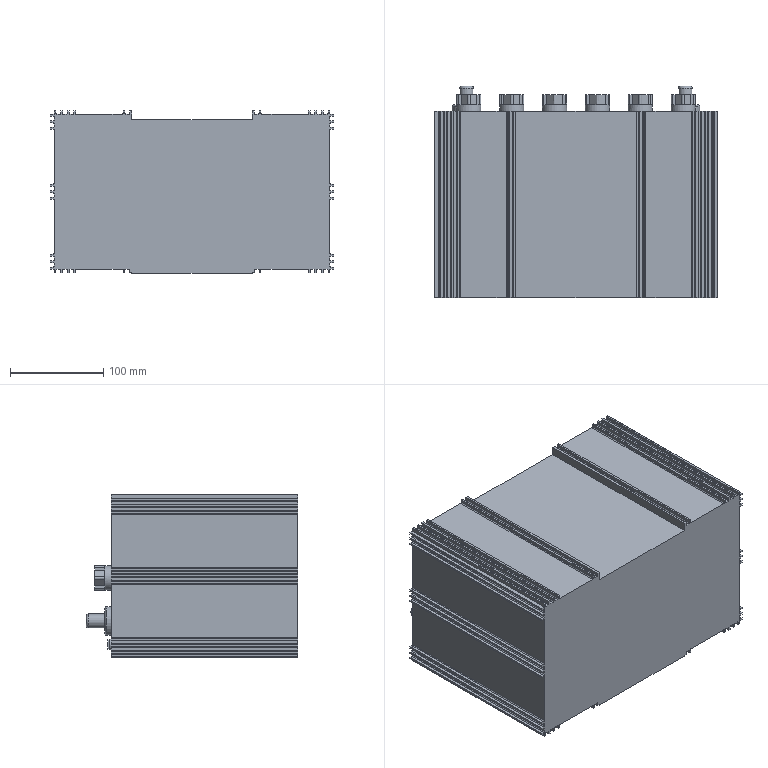Part | NX | features EXTRUDE 10, BLEND 2, DATUM_CSYS 2, SKETCH 2, EXTRACT_DATUM_PLANE 1, UNITE 1 | 1 solid | 407 faces | box 304 x 227 x 174.5 mm | volume 9929368 mm3 | plane 286 | cylinder 117 | torus 4 | commonest cylinder face diameters 2 x81 3 x24 26 x6 11.5 x2 15 x2 31 x2